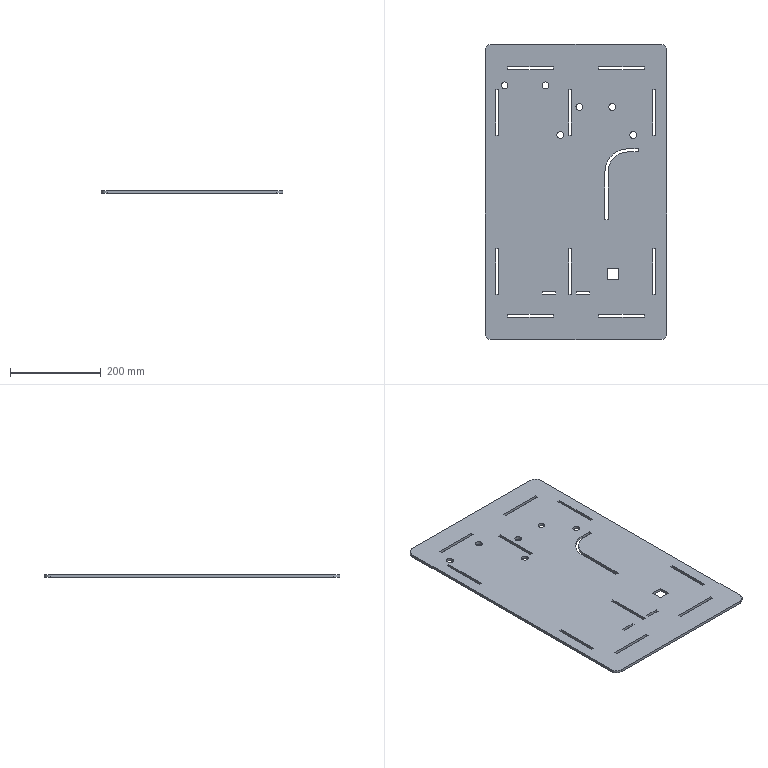Part | SolidWorks | features FlatPattern 1, SMBaseFlange 1, SheetMetal 1 | 1 solid | 82 faces | box 400 x 650 x 6 mm | volume 1502114 mm3 | plane 64 | cylinder 18 | commonest cylinder face diameters 15 x12 30 x4 87 x1 101 x1